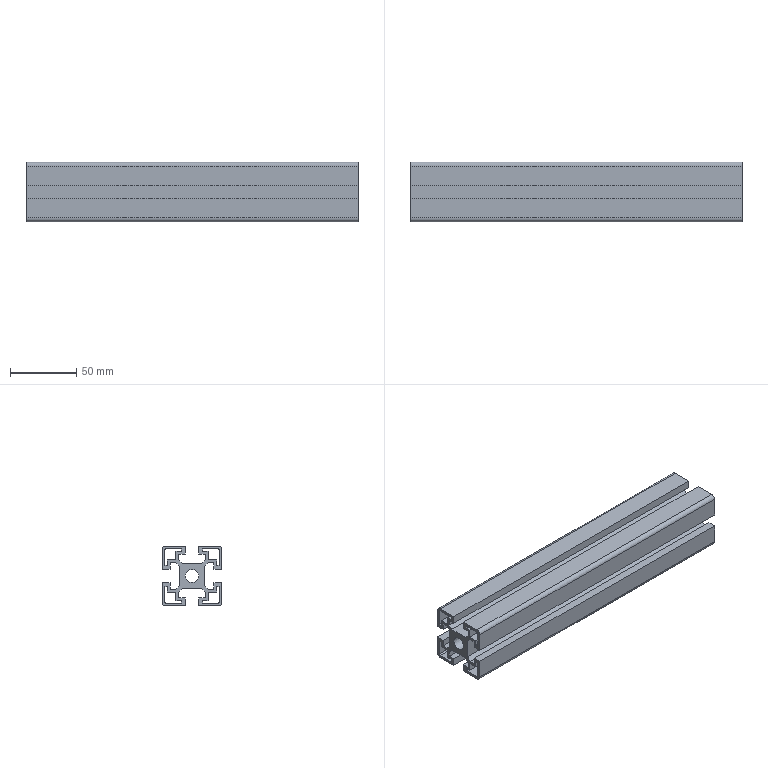Part | STEP file | 1_13 | 1 solid | 87 faces | box 250 x 45 x 45 mm | volume 204436 mm3 | plane 78 | cylinder 9 | commonest cylinder face diameters 2 x4 6 x4 10 x1